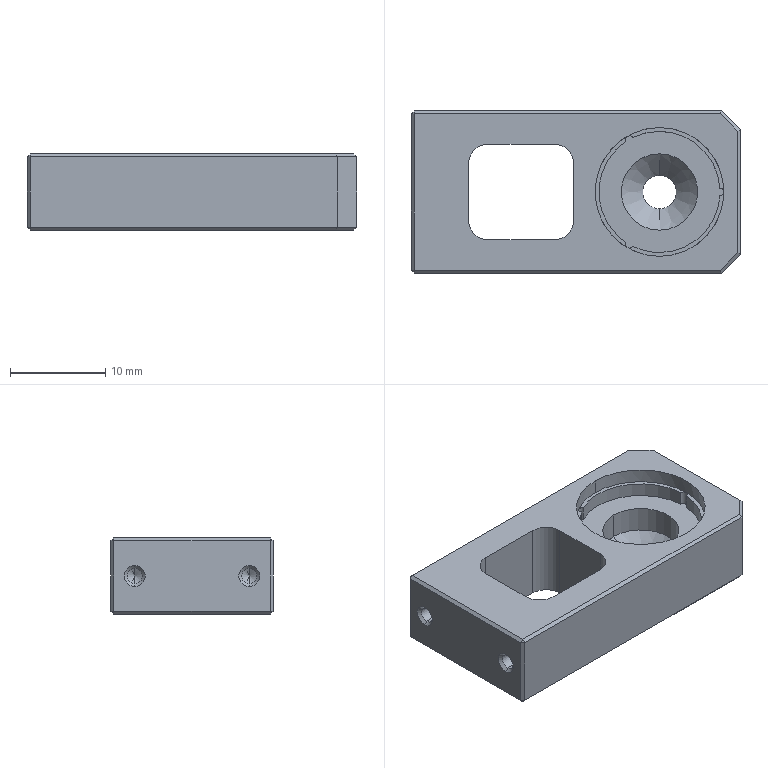NC program | NX | posted with a generic post | part box 34.5 x 17 x 8 mm
Lines 1241 to 2105 of 4112:
(ZLEVEL_PROFILE_COPY , TOOL : D3R0.5)
N2432 T08 M6
N2434 G54
N2436 G17 G0 G90 X7.053 Y1.824 S9500 M3
N2438 G43 Z30. H8
N2440 Z-1.5
N2442 G94 G1 X6.929 Y1.72 Z-1.508 F1000.
N2444 X6.772 Y1.542 Z-1.521
N2446 X6.542 Y1.176 Z-1.544
N2448 X6.443 Y0.945 Z-1.557
N2450 X6.359 Y0.739 Z-1.568
N2452 X6.259 Y0.25 Z-1.595
N2454 Y-0.25 Z-1.621
N2456 X6.359 Y-0.739 Z-1.647
N2458 X6.449 Y-0.957 Z-1.659
N2460 X6.531 Y-1.159 Z-1.671
N2462 X6.679 Y-1.406 Z-1.686
N2464 X6.821 Y-1.577 Z-1.697
N2466 X6.913 Y-1.706 Z-1.706
N2468 X6.919 Y-1.712
N2470 X7.04 Y-1.813 Z-1.714
N2472 X7.267 Y-2.003 Z-1.73
N2474 X7.537 Y-2.193 Z-1.747
N2476 X7.798 Y-2.307 Z-1.762
N2478 X8.001 Y-2.392 Z-1.774
N2480 X8.344 Y-2.473 Z-1.792
N2482 X8.694 Y-2.505 Z-1.811
N2484 X8.913 Y-2.488 Z-1.822
N2486 X9.136 Y-2.474 Z-1.834
N2488 X9.495 Y-2.391 Z-1.853
N2490 X9.702 Y-2.307 Z-1.865
N2492 X9.963 Y-2.193 Z-1.88
N2494 X10.233 Y-2.003 Z-1.897
N2496 X10.551 Y-1.737 Z-1.919
N2498 X10.709 Y-1.563 Z-1.931
N2500 X10.96 Y-1.173 Z-1.955
N2502 X11.057 Y-0.945 Z-1.968
N2504 X11.141 Y-0.739 Z-1.98
N2506 X11.241 Y-0.25 Z-2.006
N2508 Y0.25 Z-2.032
N2510 X11.141 Y0.739 Z-2.059
N2512 X11.051 Y0.957 Z-2.071
N2514 X10.969 Y1.159 Z-2.082
N2516 X10.821 Y1.406 Z-2.097
N2518 X10.679 Y1.577 Z-2.109
N2520 X10.587 Y1.706 Z-2.117
N2522 X10.581 Y1.712 Z-2.118
N2524 X10.46 Y1.813 Z-2.126
N2526 X10.233 Y2.003 Z-2.142
N2528 X9.963 Y2.193 Z-2.159
N2530 X9.702 Y2.307 Z-2.174
N2532 X9.495 Y2.391 Z-2.186
N2534 X9.136 Y2.474 Z-2.205
N2536 X8.913 Y2.488 Z-2.217
N2538 X8.694 Y2.505 Z-2.228
N2540 X8.344 Y2.473 Z-2.247
N2542 X8.001 Y2.392 Z-2.265
N2544 X7.798 Y2.307 Z-2.277
N2546 X7.537 Y2.193 Z-2.292
N2548 X7.267 Y2.003 Z-2.309
N2550 X6.929 Y1.72 Z-2.332
N2552 X6.772 Y1.542 Z-2.344
N2554 X6.542 Y1.176 Z-2.367
N2556 X6.443 Y0.945 Z-2.38
N2558 X6.359 Y0.739 Z-2.392
N2560 X6.259 Y0.25 Z-2.418
N2562 Y-0.25 Z-2.444
N2564 X6.359 Y-0.739 Z-2.47
N2566 X6.449 Y-0.957 Z-2.483
N2568 X6.531 Y-1.159 Z-2.494
N2570 X6.679 Y-1.406 Z-2.509
N2572 X6.821 Y-1.577 Z-2.521
N2574 X6.913 Y-1.706 Z-2.529
N2576 X6.919 Y-1.712 Z-2.53
N2578 X7.04 Y-1.813 Z-2.538
N2580 X7.267 Y-2.003 Z-2.553
N2582 X7.537 Y-2.193 Z-2.571
N2584 X7.798 Y-2.307 Z-2.586
N2586 X8.001 Y-2.392 Z-2.597
N2588 X8.344 Y-2.473 Z-2.616
N2590 X8.694 Y-2.505 Z-2.634
N2592 X8.913 Y-2.488 Z-2.646
N2594 X9.136 Y-2.474 Z-2.657
N2596 X9.495 Y-2.391 Z-2.677
N2598 X9.702 Y-2.307 Z-2.688
N2600 X9.963 Y-2.193 Z-2.703
N2602 X10.233 Y-2.003 Z-2.721
N2604 X10.551 Y-1.737 Z-2.742
N2606 X10.709 Y-1.563 Z-2.755
N2608 X10.96 Y-1.173 Z-2.779
N2610 X11.057 Y-0.945 Z-2.792
N2612 X11.141 Y-0.739 Z-2.804
N2614 X11.241 Y-0.25 Z-2.83
N2616 Y0.25 Z-2.856
N2618 X11.141 Y0.739 Z-2.882
N2620 X11.051 Y0.957 Z-2.894
N2622 X10.969 Y1.159 Z-2.906
N2624 X10.821 Y1.406 Z-2.921
N2626 X10.679 Y1.577 Z-2.933
N2628 X10.587 Y1.706 Z-2.941
N2630 X10.581 Y1.712
N2632 X10.46 Y1.813 Z-2.95
N2634 X10.233 Y2.003 Z-2.965
N2636 X9.963 Y2.193 Z-2.982
N2638 X9.702 Y2.307 Z-2.997
N2640 X9.495 Y2.391 Z-3.009
N2642 X9.136 Y2.474 Z-3.028
N2644 X8.913 Y2.488 Z-3.04
N2646 X8.694 Y2.505 Z-3.052
N2648 X8.344 Y2.473 Z-3.07
N2650 X8.001 Y2.392 Z-3.088
N2652 X7.798 Y2.307 Z-3.1
N2654 X7.537 Y2.193 F2000.
N2656 X7.267 Y2.003
N2658 X6.929 Y1.72
N2660 G3 X6.443 Y0.945 R2.833
N2662 X6.449 Y-0.957 R2.484
N2664 X6.821 Y-1.577 R2.387
N2666 X7.04 Y-1.813 R1.241
N2668 G1 X7.267 Y-2.003
N2670 X7.537 Y-2.193
N2672 X7.798 Y-2.307
N2674 G3 X8.913 Y-2.488 R2.41
N2676 X9.702 Y-2.307 R2.483
N2678 G1 X9.963 Y-2.193
N2680 X10.233 Y-2.003
N2682 X10.551 Y-1.737
N2684 G3 X11.057 Y-0.945 R2.756
N2686 X11.051 Y0.957 R2.484
N2688 X10.679 Y1.577 R2.386
N2690 X10.46 Y1.813 R1.241
N2692 G1 X10.233 Y2.003
N2694 X9.963 Y2.193
N2696 X9.702 Y2.307
N2698 G3 X8.913 Y2.488 R2.483
N2700 X7.798 Y2.307 R2.41
N2702 G1 X7.69 Y2.256 Z-3.102
N2704 X7.584 Y2.201 Z-3.104
N2706 X7.479 Y2.147 Z-3.106
N2708 X7.38 Y2.082 Z-3.108
N2710 X7.282 Y2.013 Z-3.11
N2712 X7.185 Y1.944 Z-3.113
N2714 X7.096 Y1.864 Z-3.115
N2716 X7.009 Y1.782 Z-3.117
N2718 X6.923 Y1.701 Z-3.119
N2720 X6.848 Y1.609 Z-3.121
N2722 X6.773 Y1.516 Z-3.123
N2724 X6.699 Y1.422 Z-3.125
N2726 X6.637 Y1.32 Z-3.127
N2728 X6.575 Y1.218 Z-3.129
N2730 X6.518 Y1.114 Z-3.131
N2732 X6.471 Y1.004 Z-3.133
N2734 X6.422 Y0.895 Z-3.135
N2736 X6.382 Y0.782 Z-3.138
N2738 X6.35 Y0.667 Z-3.14
N2740 X6.318 Y0.552 Z-3.142
N2742 X6.296 Y0.435 Z-3.144
N2744 X6.279 Y0.317 Z-3.146
N2746 X6.263 Y0.199 Z-3.148
N2748 X6.259 Y0.079 Z-3.15
N2750 Y-0.04 Z-3.152
N2752 Y-0.159 Z-3.154
N2754 X6.274 Y-0.278 Z-3.156
N2756 X6.291 Y-0.396 Z-3.158
N2758 X6.307 Y-0.514 Z-3.16
N2760 X6.34 Y-0.629 Z-3.163
N2762 X6.371 Y-0.744 Z-3.165
N2764 X6.407 Y-0.858 Z-3.167
N2766 X6.454 Y-0.968 Z-3.169
N2768 X6.502 Y-1.077 Z-3.171
N2770 X6.554 Y-1.184 Z-3.173
N2772 X6.617 Y-1.286 Z-3.175
N2774 X6.679 Y-1.388 Z-3.177
N2776 X6.747 Y-1.486 Z-3.179
N2778 X6.823 Y-1.578 Z-3.181
N2780 X6.898 Y-1.671 Z-3.183
N2782 X6.981 Y-1.756 Z-3.185
N2784 X7.068 Y-1.837 Z-3.188
N2786 X7.155 Y-1.919 Z-3.19
N2788 X7.251 Y-1.991 Z-3.192
N2790 X7.348 Y-2.06 Z-3.194
N2792 X7.446 Y-2.128 Z-3.196
N2794 X7.551 Y-2.184 Z-3.198
N2796 X7.654 Y-2.243 Z-3.2
N2798 X7.798 Y-2.307
N2800 G3 X8.913 Y-2.488 R2.404
N2802 X9.702 Y-2.307 R2.484
N2804 G1 X9.962 Y-2.193
N2806 X10.227 Y-2.007
N2808 X10.551 Y-1.737
N2810 G3 X11.057 Y-0.945 R2.758
N2812 X11.051 Y0.957 R2.484
N2814 X10.679 Y1.577 R2.386
N2816 X10.46 Y1.813 R1.24
N2818 G1 X10.227 Y2.007
N2820 X9.962 Y2.193
N2822 X9.702 Y2.307
N2824 G3 X8.913 Y2.488 R2.484
N2826 X7.798 Y2.307 R2.404
N2828 G1 X7.69 Y2.256 Z-3.202
N2830 X7.584 Y2.201 Z-3.204
N2832 X7.479 Y2.147 Z-3.206
N2834 X7.38 Y2.082 Z-3.208
N2836 X7.282 Y2.013 Z-3.21
N2838 X7.185 Y1.944 Z-3.213
N2840 X7.096 Y1.864 Z-3.215
N2842 X7.009 Y1.782 Z-3.217
N2844 X6.923 Y1.701 Z-3.219
N2846 X6.848 Y1.609 Z-3.221
N2848 X6.773 Y1.516 Z-3.223
N2850 X6.699 Y1.422 Z-3.225
N2852 X6.637 Y1.32 Z-3.227
N2854 X6.575 Y1.218 Z-3.229
N2856 X6.518 Y1.114 Z-3.231
N2858 X6.471 Y1.004 Z-3.233
N2860 X6.422 Y0.895 Z-3.235
N2862 X6.382 Y0.782 Z-3.238
N2864 X6.35 Y0.667 Z-3.24
N2866 X6.318 Y0.552 Z-3.242
N2868 X6.296 Y0.435 Z-3.244
N2870 X6.279 Y0.317 Z-3.246
N2872 X6.263 Y0.199 Z-3.248
N2874 X6.259 Y0.079 Z-3.25
N2876 Y-0.04 Z-3.252
N2878 Y-0.159 Z-3.254
N2880 X6.274 Y-0.278 Z-3.256
N2882 X6.291 Y-0.396 Z-3.258
N2884 X6.307 Y-0.514 Z-3.26
N2886 X6.34 Y-0.629 Z-3.263
N2888 X6.371 Y-0.744 Z-3.265
N2890 X6.407 Y-0.858 Z-3.267
N2892 X6.454 Y-0.968 Z-3.269
N2894 X6.502 Y-1.077 Z-3.271
N2896 X6.555 Y-1.184 Z-3.273
N2898 X6.617 Y-1.286 Z-3.275
N2900 X6.679 Y-1.388 Z-3.277
N2902 X6.747 Y-1.486 Z-3.279
N2904 X6.823 Y-1.578 Z-3.281
N2906 X6.898 Y-1.671 Z-3.283
N2908 X6.981 Y-1.756 Z-3.285
N2910 X7.068 Y-1.837 Z-3.288
N2912 X7.155 Y-1.919 Z-3.29
N2914 X7.251 Y-1.991 Z-3.292
N2916 X7.349 Y-2.06 Z-3.294
N2918 X7.446 Y-2.128 Z-3.296
N2920 X7.551 Y-2.184 Z-3.298
N2922 X7.654 Y-2.243 Z-3.3
N2924 X7.798 Y-2.307
N2926 G3 X8.918 Y-2.488 R2.409
N2928 X9.702 Y-2.307 R2.456
N2930 G1 X9.96 Y-2.193
N2932 X10.222 Y-2.011
N2934 X10.55 Y-1.738
N2936 G3 X11.057 Y-0.945 R2.759
N2938 X11.051 Y0.957 R2.484
N2940 X10.679 Y1.577 R2.386
N2942 X10.46 Y1.813 R1.239
N2944 G1 X10.222 Y2.011
N2946 X9.96 Y2.193
N2948 X9.702 Y2.307
N2950 G3 X8.918 Y2.488 R2.456
N2952 X7.798 Y2.307 R2.409
N2954 G1 X7.69 Y2.256 Z-3.302
N2956 X7.584 Y2.201 Z-3.304
N2958 X7.479 Y2.147 Z-3.306
N2960 X7.38 Y2.082 Z-3.308
N2962 X7.282 Y2.013 Z-3.31
N2964 X7.184 Y1.944 Z-3.313
N2966 X7.096 Y1.864 Z-3.315
N2968 X7.009 Y1.782 Z-3.317
N2970 X6.923 Y1.701 Z-3.319
N2972 X6.847 Y1.609 Z-3.321
N2974 X6.772 Y1.516 Z-3.323
N2976 X6.699 Y1.422 Z-3.325
N2978 X6.637 Y1.32 Z-3.327
N2980 X6.575 Y1.218 Z-3.329
N2982 X6.518 Y1.114 Z-3.331
N2984 X6.471 Y1.004 Z-3.333
N2986 X6.423 Y0.895 Z-3.335
N2988 X6.382 Y0.782 Z-3.338
N2990 X6.35 Y0.667 Z-3.34
N2992 X6.318 Y0.552 Z-3.342
N2994 X6.296 Y0.435 Z-3.344
N2996 X6.279 Y0.317 Z-3.346
N2998 X6.263 Y0.199 Z-3.348
N3000 X6.259 Y0.079 Z-3.35
N3002 Y-0.04 Z-3.352
N3004 Y-0.159 Z-3.354
N3006 X6.274 Y-0.278 Z-3.356
N3008 X6.291 Y-0.396 Z-3.358
N3010 X6.307 Y-0.514 Z-3.36
N3012 X6.34 Y-0.629 Z-3.363
N3014 X6.371 Y-0.744 Z-3.365
N3016 X6.407 Y-0.858 Z-3.367
N3018 X6.455 Y-0.968 Z-3.369
N3020 X6.502 Y-1.077 Z-3.371
N3022 X6.555 Y-1.184 Z-3.373
N3024 X6.617 Y-1.286 Z-3.375
N3026 X6.679 Y-1.388 Z-3.377
N3028 X6.747 Y-1.486 Z-3.379
N3030 X6.823 Y-1.578 Z-3.381
N3032 X6.898 Y-1.671 Z-3.383
N3034 X6.981 Y-1.756 Z-3.385
N3036 X7.068 Y-1.837 Z-3.388
N3038 X7.155 Y-1.919 Z-3.39
N3040 X7.251 Y-1.991 Z-3.392
N3042 X7.349 Y-2.06 Z-3.394
N3044 X7.446 Y-2.129 Z-3.396
N3046 X7.551 Y-2.184 Z-3.398
N3048 X7.654 Y-2.243 Z-3.4
N3050 X7.798 Y-2.307
N3052 G3 X8.918 Y-2.488 R2.404
N3054 X9.702 Y-2.307 R2.458
N3056 G1 X9.959 Y-2.194
N3058 X10.217 Y-2.015
N3060 X10.55 Y-1.739
N3062 G3 X11.057 Y-0.945 R2.761
N3064 X11.051 Y0.957 R2.484
N3066 X10.679 Y1.577 R2.386
N3068 X10.46 Y1.813 R1.238
N3070 G1 X10.217 Y2.015
N3072 X9.959 Y2.194
N3074 X9.702 Y2.307
N3076 G3 X8.918 Y2.488 R2.458
N3078 X7.798 Y2.307 R2.404
N3080 G1 X7.69 Y2.256 Z-3.402
N3082 X7.584 Y2.201 Z-3.404
N3084 X7.479 Y2.147 Z-3.406
N3086 X7.38 Y2.082 Z-3.408
N3088 X7.282 Y2.013 Z-3.41
N3090 X7.185 Y1.943 Z-3.413
N3092 X7.096 Y1.864 Z-3.415
N3094 X7.009 Y1.782 Z-3.417
N3096 X6.923 Y1.701 Z-3.419
N3098 X6.848 Y1.609 Z-3.421
N3100 X6.772 Y1.516 Z-3.423
N3102 X6.7 Y1.422 Z-3.425
N3104 X6.637 Y1.32 Z-3.427
N3106 X6.576 Y1.218 Z-3.429
N3108 X6.518 Y1.113 Z-3.431
N3110 X6.47 Y1.004 Z-3.433
N3112 X6.423 Y0.894 Z-3.435
N3114 X6.383 Y0.782 Z-3.438
N3116 X6.35 Y0.667 Z-3.44
N3118 X6.318 Y0.552 Z-3.442
N3120 X6.296 Y0.435 Z-3.444
N3122 X6.28 Y0.317 Z-3.446
N3124 X6.263 Y0.199 Z-3.448
N3126 X6.26 Y0.079 Z-3.45
N3128 X6.259 Y-0.04 Z-3.452
N3130 Y-0.159 Z-3.454
N3132 X6.274 Y-0.278 Z-3.456
N3134 X6.29 Y-0.396 Z-3.458
N3136 X6.307 Y-0.514 Z-3.46
N3138 X6.339 Y-0.629 Z-3.463
N3140 X6.372 Y-0.744 Z-3.465
N3142 X6.407 Y-0.858 Z-3.467
N3144 X6.455 Y-0.968 Z-3.469
N3146 X6.502 Y-1.077 Z-3.471
N3148 X6.555 Y-1.184 Z-3.473
N3150 X6.617 Y-1.286 Z-3.475
N3152 X6.679 Y-1.388 Z-3.477
N3154 X6.748 Y-1.486 Z-3.479
N3156 X6.823 Y-1.578 Z-3.481
N3158 X6.898 Y-1.671 Z-3.483
N3160 X6.981 Y-1.756 Z-3.485
N3162 X7.068 Y-1.838 Z-3.488
N3164 X7.156 Y-1.919 Z-3.49
N3166 X7.251 Y-1.991 Z-3.492
N3168 X7.349 Y-2.06 Z-3.494
N3170 X7.447 Y-2.128 Z-3.496
N3172 X7.551 Y-2.185 Z-3.498
N3174 X7.653 Y-2.246 Z-3.5
N3176 G3 X7.797 Y2.311 R-2.5
N3178 G1 X7.691 Y2.256 Z-3.502
N3180 X7.585 Y2.202 Z-3.504
N3182 X7.479 Y2.147 Z-3.506
N3184 X7.38 Y2.081 Z-3.508
N3186 X7.282 Y2.013 Z-3.51
N3188 X7.185 Y1.944 Z-3.513
N3190 X7.097 Y1.864 Z-3.515
N3192 X7.01 Y1.783 Z-3.517
N3194 X6.923 Y1.701 Z-3.519
N3196 X6.848 Y1.609 Z-3.521
N3198 X6.773 Y1.517 Z-3.523
N3200 X6.7 Y1.422 Z-3.525
N3202 X6.638 Y1.321 Z-3.527
N3204 X6.577 Y1.219 Z-3.529
N3206 X6.519 Y1.115 Z-3.531
N3208 X6.471 Y1.006 Z-3.533
N3210 X6.424 Y0.897 Z-3.535
N3212 X6.383 Y0.785 Z-3.538
N3214 X6.351 Y0.67 Z-3.54
N3216 X6.319 Y0.556 Z-3.542
N3218 X6.296 Y0.439 Z-3.544
N3220 X6.28 Y0.321 Z-3.546
N3222 X6.263 Y0.203 Z-3.548
N3224 X6.26 Y0.084 Z-3.55
N3226 X6.259 Y-0.035 Z-3.552
N3228 Y-0.154 Z-3.554
N3230 X6.273 Y-0.272 Z-3.556
N3232 X6.29 Y-0.39 Z-3.558
N3234 X6.306 Y-0.508 Z-3.56
N3236 X6.338 Y-0.623 Z-3.563
N3238 X6.37 Y-0.738 Z-3.565
N3240 X6.404 Y-0.852 Z-3.567
N3242 X6.452 Y-0.961 Z-3.569
N3244 X6.499 Y-1.07 Z-3.571
N3246 X6.55 Y-1.177 Z-3.573
N3248 X6.612 Y-1.279 Z-3.575
N3250 X6.674 Y-1.381 Z-3.577
N3252 X6.742 Y-1.479 Z-3.579
N3254 X6.817 Y-1.571 Z-3.581
N3256 X6.892 Y-1.663 Z-3.583
N3258 X6.974 Y-1.75 Z-3.585
N3260 X7.061 Y-1.831 Z-3.588
N3262 X7.148 Y-1.912 Z-3.59
N3264 X7.243 Y-1.984 Z-3.592
N3266 X7.34 Y-2.053 Z-3.594
N3268 X7.437 Y-2.122 Z-3.596
N3270 X7.541 Y-2.179 Z-3.598
N3272 X7.643 Y-2.242 Z-3.6
N3274 G3 X7.797 Y2.311 R-2.5
N3276 G1 X7.691 Y2.256 Z-3.602
N3278 X7.585 Y2.202 Z-3.604
N3280 X7.479 Y2.147 Z-3.606
N3282 X7.38 Y2.081 Z-3.608
N3284 X7.282 Y2.013 Z-3.61
N3286 X7.185 Y1.944 Z-3.613
N3288 X7.097 Y1.864 Z-3.615
N3290 X7.01 Y1.783 Z-3.617
N3292 X6.923 Y1.701 Z-3.619
N3294 X6.848 Y1.609 Z-3.621
N3296 X6.773 Y1.517 Z-3.623
N3298 X6.7 Y1.422 Z-3.625
N3300 X6.638 Y1.321 Z-3.627
N3302 X6.577 Y1.219 Z-3.629
N3304 X6.519 Y1.115 Z-3.631
N3306 X6.471 Y1.006 Z-3.633
N3308 X6.424 Y0.897 Z-3.635
N3310 X6.383 Y0.785 Z-3.638
N3312 X6.351 Y0.67 Z-3.64
N3314 X6.319 Y0.556 Z-3.642
N3316 X6.296 Y0.439 Z-3.644
N3318 X6.28 Y0.321 Z-3.646
N3320 X6.263 Y0.203 Z-3.648
N3322 X6.26 Y0.084 Z-3.65
N3324 X6.259 Y-0.035 Z-3.652
N3326 Y-0.154 Z-3.654
N3328 X6.273 Y-0.272 Z-3.656
N3330 X6.29 Y-0.39 Z-3.658
N3332 X6.305 Y-0.508 Z-3.66
N3334 X6.338 Y-0.623 Z-3.663
N3336 X6.37 Y-0.738 Z-3.665
N3338 X6.404 Y-0.852 Z-3.667
N3340 X6.452 Y-0.961 Z-3.669
N3342 X6.499 Y-1.07 Z-3.671
N3344 X6.55 Y-1.177 Z-3.673
N3346 X6.612 Y-1.279 Z-3.675
N3348 X6.674 Y-1.381 Z-3.677
N3350 X6.742 Y-1.479 Z-3.679
N3352 X6.817 Y-1.571 Z-3.681
N3354 X6.892 Y-1.663 Z-3.683
N3356 X6.974 Y-1.75 Z-3.685
N3358 X7.061 Y-1.831 Z-3.688
N3360 X7.148 Y-1.912 Z-3.69
N3362 X7.243 Y-1.984 Z-3.692
N3364 X7.34 Y-2.053 Z-3.694
N3366 X7.437 Y-2.122 Z-3.696
N3368 X7.541 Y-2.179 Z-3.698
N3370 X7.643 Y-2.242 Z-3.7
N3372 G3 X7.797 Y2.311 R-2.5
N3374 G1 X7.691 Y2.256 Z-3.702
N3376 X7.585 Y2.202 Z-3.704
N3378 X7.479 Y2.147 Z-3.706
N3380 X7.38 Y2.081 Z-3.708
N3382 X7.282 Y2.013 Z-3.71
N3384 X7.185 Y1.944 Z-3.713
N3386 X7.097 Y1.864 Z-3.715
N3388 X7.01 Y1.783 Z-3.717
N3390 X6.923 Y1.701 Z-3.719
N3392 X6.848 Y1.609 Z-3.721
N3394 X6.773 Y1.517 Z-3.723
N3396 X6.7 Y1.422 Z-3.725
N3398 X6.638 Y1.321 Z-3.727
N3400 X6.577 Y1.219 Z-3.729
N3402 X6.519 Y1.115 Z-3.731
N3404 X6.471 Y1.006 Z-3.733
N3406 X6.424 Y0.897 Z-3.735
N3408 X6.383 Y0.785 Z-3.738
N3410 X6.351 Y0.67 Z-3.74
N3412 X6.319 Y0.556 Z-3.742
N3414 X6.296 Y0.439 Z-3.744
N3416 X6.28 Y0.321 Z-3.746
N3418 X6.263 Y0.203 Z-3.748
N3420 X6.26 Y0.084 Z-3.75
N3422 X6.259 Y-0.035 Z-3.752
N3424 Y-0.154 Z-3.754
N3426 X6.273 Y-0.272 Z-3.756
N3428 X6.29 Y-0.39 Z-3.758
N3430 X6.305 Y-0.508 Z-3.76
N3432 X6.338 Y-0.623 Z-3.763
N3434 X6.37 Y-0.738 Z-3.765
N3436 X6.404 Y-0.852 Z-3.767
N3438 X6.452 Y-0.961 Z-3.769
N3440 X6.499 Y-1.07 Z-3.771
N3442 X6.55 Y-1.177 Z-3.773
N3444 X6.613 Y-1.279 Z-3.775
N3446 X6.674 Y-1.381 Z-3.777
N3448 X6.742 Y-1.479 Z-3.779
N3450 X6.817 Y-1.571 Z-3.781
N3452 X6.892 Y-1.663 Z-3.783
N3454 X6.974 Y-1.75 Z-3.785
N3456 X7.061 Y-1.831 Z-3.788
N3458 X7.148 Y-1.912 Z-3.79
N3460 X7.243 Y-1.984 Z-3.792
N3462 X7.34 Y-2.053 Z-3.794
N3464 X7.437 Y-2.122 Z-3.796
N3466 X7.541 Y-2.179 Z-3.798
N3468 X7.643 Y-2.242 Z-3.8
N3470 G3 X7.797 Y2.311 R-2.5
N3472 G1 X7.691 Y2.256 Z-3.802
N3474 X7.585 Y2.202 Z-3.804
N3476 X7.479 Y2.147 Z-3.806
N3478 X7.38 Y2.081 Z-3.808
N3480 X7.282 Y2.013 Z-3.81
N3482 X7.185 Y1.944 Z-3.813
N3484 X7.097 Y1.864 Z-3.815
N3486 X7.01 Y1.783 Z-3.817
N3488 X6.923 Y1.701 Z-3.819
N3490 X6.848 Y1.609 Z-3.821
N3492 X6.773 Y1.517 Z-3.823
N3494 X6.7 Y1.422 Z-3.825
N3496 X6.638 Y1.321 Z-3.827
N3498 X6.577 Y1.219 Z-3.829
N3500 X6.519 Y1.115 Z-3.831
N3502 X6.471 Y1.006 Z-3.833
N3504 X6.424 Y0.897 Z-3.835
N3506 X6.383 Y0.785 Z-3.838
N3508 X6.351 Y0.67 Z-3.84
N3510 X6.319 Y0.556 Z-3.842
N3512 X6.296 Y0.439 Z-3.844
N3514 X6.28 Y0.321 Z-3.846
N3516 X6.264 Y0.203 Z-3.848
N3518 X6.26 Y0.084 Z-3.85
N3520 X6.259 Y-0.035 Z-3.852
N3522 Y-0.154 Z-3.854
N3524 X6.273 Y-0.272 Z-3.856
N3526 X6.29 Y-0.39 Z-3.858
N3528 X6.305 Y-0.508 Z-3.86
N3530 X6.338 Y-0.623 Z-3.863
N3532 X6.37 Y-0.738 Z-3.865
N3534 X6.404 Y-0.852 Z-3.867
N3536 X6.452 Y-0.961 Z-3.869
N3538 X6.499 Y-1.07 Z-3.871
N3540 X6.551 Y-1.177 Z-3.873
N3542 X6.613 Y-1.279 Z-3.875
N3544 X6.674 Y-1.381 Z-3.877
N3546 X6.742 Y-1.479 Z-3.879
N3548 X6.817 Y-1.571 Z-3.881
N3550 X6.892 Y-1.663 Z-3.883
N3552 X6.974 Y-1.75 Z-3.885
N3554 X7.061 Y-1.831 Z-3.888
N3556 X7.148 Y-1.912 Z-3.89
N3558 X7.243 Y-1.984 Z-3.892
N3560 X7.34 Y-2.053 Z-3.894
N3562 X7.437 Y-2.122 Z-3.896
N3564 X7.541 Y-2.179 Z-3.898
N3566 X7.643 Y-2.242 Z-3.9
N3568 G3 X7.797 Y2.311 R-2.5
N3570 G1 X7.691 Y2.256 Z-3.902
N3572 X7.585 Y2.202 Z-3.904
N3574 X7.479 Y2.147 Z-3.906
N3576 X7.38 Y2.081 Z-3.908
N3578 X7.282 Y2.013 Z-3.91
N3580 X7.185 Y1.944 Z-3.913
N3582 X7.097 Y1.864 Z-3.915
N3584 X7.01 Y1.783 Z-3.917
N3586 X6.923 Y1.701 Z-3.919
N3588 X6.848 Y1.609 Z-3.921
N3590 X6.773 Y1.517 Z-3.923
N3592 X6.7 Y1.422 Z-3.925
N3594 X6.638 Y1.321 Z-3.927
N3596 X6.577 Y1.219 Z-3.929
N3598 X6.519 Y1.115 Z-3.931
N3600 X6.471 Y1.006 Z-3.933
N3602 X6.424 Y0.897 Z-3.935
N3604 X6.383 Y0.785 Z-3.938
N3606 X6.351 Y0.67 Z-3.94
N3608 X6.319 Y0.556 Z-3.942
N3610 X6.296 Y0.439 Z-3.944
N3612 X6.28 Y0.321 Z-3.946
N3614 X6.264 Y0.203 Z-3.948
N3616 X6.26 Y0.084 Z-3.95
N3618 X6.259 Y-0.035 Z-3.952
N3620 Y-0.154 Z-3.954
N3622 X6.273 Y-0.272 Z-3.956
N3624 X6.29 Y-0.39 Z-3.958
N3626 X6.305 Y-0.508 Z-3.96
N3628 X6.338 Y-0.623 Z-3.963
N3630 X6.37 Y-0.738 Z-3.965
N3632 X6.404 Y-0.852 Z-3.967
N3634 X6.451 Y-0.961 Z-3.969
N3636 X6.499 Y-1.07 Z-3.971
N3638 X6.551 Y-1.177 Z-3.973
N3640 X6.613 Y-1.279 Z-3.975
N3642 X6.674 Y-1.381 Z-3.977
N3644 X6.742 Y-1.479 Z-3.979
N3646 X6.817 Y-1.571 Z-3.981
N3648 X6.892 Y-1.663 Z-3.983
N3650 X6.974 Y-1.75 Z-3.985
N3652 X7.061 Y-1.831 Z-3.988
N3654 X7.148 Y-1.912 Z-3.99
N3656 X7.243 Y-1.984 Z-3.992
N3658 X7.34 Y-2.053 Z-3.994
N3660 X7.437 Y-2.122 Z-3.996
N3662 X7.541 Y-2.179 Z-3.998
N3664 X7.643 Y-2.242 Z-4.
N3666 G3 X7.797 Y2.311 R-2.5
N3668 G1 X7.691 Y2.256 Z-4.002
N3670 X7.585 Y2.202 Z-4.004
N3672 X7.479 Y2.147 Z-4.006
N3674 X7.38 Y2.081 Z-4.008
N3676 X7.282 Y2.013 Z-4.01
N3678 X7.185 Y1.944 Z-4.013
N3680 X7.097 Y1.864 Z-4.015
N3682 X7.01 Y1.783 Z-4.017
N3684 X6.923 Y1.701 Z-4.019
N3686 X6.848 Y1.609 Z-4.021
N3688 X6.773 Y1.517 Z-4.023
N3690 X6.7 Y1.422 Z-4.025
N3692 X6.638 Y1.321 Z-4.027
N3694 X6.577 Y1.219 Z-4.029
N3696 X6.518 Y1.115 Z-4.031
N3698 X6.471 Y1.006 Z-4.033
N3700 X6.424 Y0.897 Z-4.035
N3702 X6.383 Y0.785 Z-4.038
N3704 X6.351 Y0.67 Z-4.04
N3706 X6.319 Y0.556 Z-4.042
N3708 X6.296 Y0.439 Z-4.044
N3710 X6.28 Y0.321 Z-4.046
N3712 X6.264 Y0.203 Z-4.048
N3714 X6.26 Y0.084 Z-4.05
N3716 X6.259 Y-0.035 Z-4.052
N3718 Y-0.154 Z-4.054
N3720 X6.273 Y-0.272 Z-4.056
N3722 X6.29 Y-0.39 Z-4.058
N3724 X6.305 Y-0.508 Z-4.06
N3726 X6.338 Y-0.623 Z-4.063
N3728 X6.37 Y-0.738 Z-4.065
N3730 X6.404 Y-0.852 Z-4.067
N3732 X6.451 Y-0.961 Z-4.069
N3734 X6.5 Y-1.07 Z-4.071
N3736 X6.551 Y-1.177 Z-4.073
N3738 X6.613 Y-1.279 Z-4.075
N3740 X6.674 Y-1.381 Z-4.077
N3742 X6.742 Y-1.479 Z-4.079
N3744 X6.817 Y-1.571 Z-4.081
N3746 X6.892 Y-1.663 Z-4.083
N3748 X6.974 Y-1.75 Z-4.085
N3750 X7.061 Y-1.831 Z-4.088
N3752 X7.148 Y-1.912 Z-4.09
N3754 X7.243 Y-1.984 Z-4.092
N3756 X7.339 Y-2.053 Z-4.094
N3758 X7.437 Y-2.122 Z-4.096
N3760 X7.541 Y-2.179 Z-4.098
N3762 X7.643 Y-2.242 Z-4.1
N3764 G3 X7.797 Y2.311 R-2.5
N3766 G1 X7.69 Y2.257 Z-4.102
N3768 X7.585 Y2.202 Z-4.104
N3770 X7.479 Y2.147 Z-4.106
N3772 X7.38 Y2.081 Z-4.108
N3774 X7.282 Y2.013 Z-4.11
N3776 X7.185 Y1.944 Z-4.113
N3778 X7.097 Y1.864 Z-4.115
N3780 X7.01 Y1.783 Z-4.117
N3782 X6.923 Y1.701 Z-4.119
N3784 X6.848 Y1.609 Z-4.121
N3786 X6.773 Y1.517 Z-4.123
N3788 X6.7 Y1.422 Z-4.125
N3790 X6.638 Y1.321 Z-4.127
N3792 X6.577 Y1.219 Z-4.129
N3794 X6.518 Y1.115 Z-4.131
N3796 X6.471 Y1.006 Z-4.133
N3798 X6.424 Y0.897 Z-4.135
N3800 X6.383 Y0.785 Z-4.138
N3802 X6.351 Y0.67 Z-4.14
N3804 X6.319 Y0.556 Z-4.142
N3806 X6.296 Y0.439 Z-4.144
N3808 X6.28 Y0.321 Z-4.146
N3810 X6.264 Y0.203 Z-4.148
N3812 X6.26 Y0.084 Z-4.15
N3814 X6.259 Y-0.035 Z-4.152
N3816 Y-0.154 Z-4.154
N3818 X6.273 Y-0.272 Z-4.156
N3820 X6.29 Y-0.39 Z-4.158
N3822 X6.306 Y-0.508 Z-4.16
N3824 X6.338 Y-0.623 Z-4.163
N3826 X6.37 Y-0.738 Z-4.165
N3828 X6.404 Y-0.852 Z-4.167
N3830 X6.451 Y-0.961 Z-4.169
N3832 X6.5 Y-1.07 Z-4.171
N3834 X6.551 Y-1.177 Z-4.173
N3836 X6.613 Y-1.279 Z-4.175
N3838 X6.674 Y-1.381 Z-4.177
N3840 X6.742 Y-1.479 Z-4.179
N3842 X6.817 Y-1.571 Z-4.181
N3844 X6.892 Y-1.663 Z-4.183
N3846 X6.974 Y-1.749 Z-4.185
N3848 X7.061 Y-1.831 Z-4.188
N3850 X7.148 Y-1.912 Z-4.19
N3852 X7.243 Y-1.984 Z-4.192
N3854 X7.339 Y-2.053 Z-4.194
N3856 X7.437 Y-2.122 Z-4.196
N3858 X7.541 Y-2.179 Z-4.198
N3860 X7.643 Y-2.242 Z-4.2
N3862 G3 X7.797 Y2.311 R-2.5
N3864 G1 X7.691 Y2.257 Z-4.202
N3866 X7.585 Y2.201 Z-4.204
N3868 X7.479 Y2.147 Z-4.206
N3870 X7.38 Y2.081 Z-4.208
N3872 X7.282 Y2.013 Z-4.21
N3874 X7.185 Y1.944 Z-4.213
N3876 X7.097 Y1.864 Z-4.215
N3878 X7.01 Y1.783 Z-4.217
N3880 X6.923 Y1.701 Z-4.219
N3882 X6.848 Y1.609 Z-4.221
N3884 X6.773 Y1.517 Z-4.223
N3886 X6.7 Y1.422 Z-4.225
N3888 X6.638 Y1.321 Z-4.227
N3890 X6.577 Y1.219 Z-4.229
N3892 X6.518 Y1.115 Z-4.231
N3894 X6.471 Y1.006 Z-4.233
N3896 X6.424 Y0.897 Z-4.235
N3898 X6.383 Y0.785 Z-4.238
N3900 X6.351 Y0.67 Z-4.24
N3902 X6.319 Y0.556 Z-4.242
N3904 X6.296 Y0.439 Z-4.244
N3906 X6.28 Y0.321 Z-4.246
N3908 X6.264 Y0.203 Z-4.248
N3910 X6.26 Y0.084 Z-4.25
N3912 X6.259 Y-0.035 Z-4.252
N3914 Y-0.154 Z-4.254
N3916 X6.273 Y-0.272 Z-4.256
N3918 X6.29 Y-0.39 Z-4.258
N3920 X6.306 Y-0.508 Z-4.26
N3922 X6.338 Y-0.623 Z-4.263
N3924 X6.37 Y-0.738 Z-4.265
N3926 X6.404 Y-0.852 Z-4.267
N3928 X6.452 Y-0.961 Z-4.269
N3930 X6.5 Y-1.07 Z-4.271
N3932 X6.551 Y-1.177 Z-4.273
N3934 X6.613 Y-1.279 Z-4.275
N3936 X6.674 Y-1.381 Z-4.277
N3938 X6.742 Y-1.479 Z-4.279
N3940 X6.817 Y-1.571 Z-4.281
N3942 X6.892 Y-1.663 Z-4.283
N3944 X6.974 Y-1.749 Z-4.285
N3946 X7.061 Y-1.831 Z-4.288
N3948 X7.148 Y-1.912 Z-4.29
N3950 X7.243 Y-1.984 Z-4.292
N3952 X7.339 Y-2.053 Z-4.294
N3954 X7.437 Y-2.122 Z-4.296
N3956 X7.541 Y-2.179 Z-4.298
N3958 X7.643 Y-2.242 Z-4.3
N3960 G3 X7.797 Y2.311 R-2.5
N3962 G1 X7.691 Y2.257 Z-4.302
N3964 X7.585 Y2.201 Z-4.304
N3966 X7.479 Y2.147 Z-4.306
N3968 X7.38 Y2.081 Z-4.308
N3970 X7.282 Y2.013 Z-4.31
N3972 X7.185 Y1.944 Z-4.313
N3974 X7.097 Y1.864 Z-4.315
N3976 X7.01 Y1.783 Z-4.317
N3978 X6.923 Y1.701 Z-4.319
N3980 X6.848 Y1.609 Z-4.321
N3982 X6.773 Y1.517 Z-4.323
N3984 X6.7 Y1.422 Z-4.325
N3986 X6.638 Y1.321 Z-4.327
N3988 X6.577 Y1.219 Z-4.329
N3990 X6.519 Y1.115 Z-4.331
N3992 X6.471 Y1.006 Z-4.333
N3994 X6.424 Y0.896 Z-4.335
N3996 X6.383 Y0.785 Z-4.338
N3998 X6.351 Y0.67 Z-4.34
N4000 X6.319 Y0.556 Z-4.342
N4002 X6.296 Y0.439 Z-4.344
N4004 X6.28 Y0.321 Z-4.346
N4006 X6.264 Y0.203 Z-4.348
N4008 X6.26 Y0.084 Z-4.35
N4010 X6.259 Y-0.035 Z-4.352
N4012 Y-0.154 Z-4.354
N4014 X6.273 Y-0.272 Z-4.356
N4016 X6.29 Y-0.39 Z-4.358
N4018 X6.306 Y-0.508 Z-4.36
N4020 X6.338 Y-0.623 Z-4.363
N4022 X6.37 Y-0.738 Z-4.365
N4024 X6.404 Y-0.852 Z-4.367
N4026 X6.452 Y-0.961 Z-4.369
N4028 X6.5 Y-1.07 Z-4.371
N4030 X6.551 Y-1.177 Z-4.373
N4032 X6.613 Y-1.279 Z-4.375
N4034 X6.674 Y-1.381 Z-4.377
N4036 X6.742 Y-1.479 Z-4.379
N4038 X6.817 Y-1.571 Z-4.381
N4040 X6.892 Y-1.663 Z-4.383
N4042 X6.974 Y-1.749 Z-4.385
N4044 X7.061 Y-1.831 Z-4.388
N4046 X7.148 Y-1.912 Z-4.39
N4048 X7.243 Y-1.984 Z-4.392
N4050 X7.34 Y-2.053 Z-4.394
N4052 X7.437 Y-2.122 Z-4.396
N4054 X7.542 Y-2.179 Z-4.398
N4056 X7.643 Y-2.242 Z-4.4
N4058 G3 X7.797 Y2.311 R-2.5
N4060 G1 X7.691 Y2.257 Z-4.402
N4062 X7.585 Y2.201 Z-4.404
N4064 X7.479 Y2.147 Z-4.406
N4066 X7.38 Y2.081 Z-4.408
N4068 X7.282 Y2.013 Z-4.41
N4070 X7.185 Y1.944 Z-4.413
N4072 X7.097 Y1.864 Z-4.415
N4074 X7.01 Y1.783 Z-4.417
N4076 X6.923 Y1.701 Z-4.419
N4078 X6.848 Y1.609 Z-4.421
N4080 X6.773 Y1.516 Z-4.423
N4082 X6.7 Y1.422 Z-4.425
N4084 X6.638 Y1.321 Z-4.427
N4086 X6.577 Y1.219 Z-4.429
N4088 X6.519 Y1.115 Z-4.431
N4090 X6.471 Y1.006 Z-4.433
N4092 X6.424 Y0.896 Z-4.435
N4094 X6.383 Y0.785 Z-4.438
N4096 X6.351 Y0.67 Z-4.44
N4098 X6.319 Y0.556 Z-4.442
N4100 X6.296 Y0.439 Z-4.444
N4102 X6.28 Y0.321 Z-4.446
N4104 X6.264 Y0.203 Z-4.448
N4106 X6.26 Y0.084 Z-4.45
N4108 X6.259 Y-0.035 Z-4.452
N4110 Y-0.154 Z-4.454
N4112 X6.273 Y-0.272 Z-4.456
N4114 X6.29 Y-0.39 Z-4.458
N4116 X6.306 Y-0.508 Z-4.46
N4118 X6.338 Y-0.623 Z-4.463
N4120 X6.37 Y-0.738 Z-4.465
N4122 X6.404 Y-0.852 Z-4.467
N4124 X6.452 Y-0.961 Z-4.469
N4126 X6.5 Y-1.07 Z-4.471
N4128 X6.551 Y-1.177 Z-4.473
N4130 X6.613 Y-1.279 Z-4.475
N4132 X6.674 Y-1.381 Z-4.477
N4134 X6.742 Y-1.479 Z-4.479
N4136 X6.817 Y-1.571 Z-4.481
N4138 X6.892 Y-1.663 Z-4.483
N4140 X6.974 Y-1.749 Z-4.485
N4142 X7.061 Y-1.831 Z-4.488
N4144 X7.148 Y-1.912 Z-4.49
N4146 X7.243 Y-1.984 Z-4.492
N4148 X7.34 Y-2.053 Z-4.494
N4150 X7.437 Y-2.122 Z-4.496
N4152 X7.542 Y-2.179 Z-4.498
N4154 X7.643 Y-2.242 Z-4.5